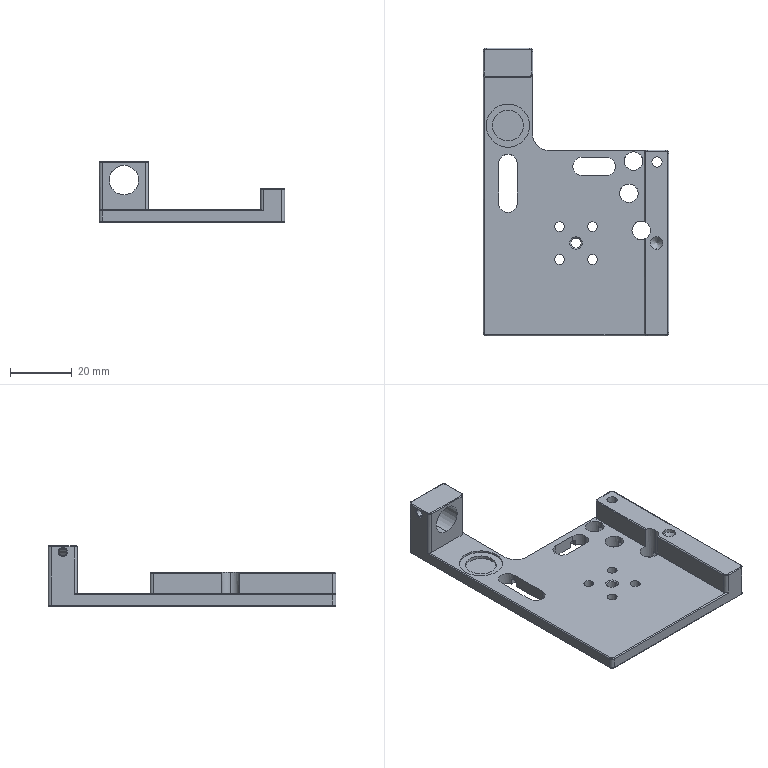Part | STEP file | 1 solid | 148 faces | box 60 x 93 x 19.5 mm | volume 19788 mm3 | cylinder 74 | plane 49 | torus 15 | cone 10 | commonest cylinder face diameters 2 x23 0.6 x17 6 x11 3.2 x8 3.3 x4 10 x3